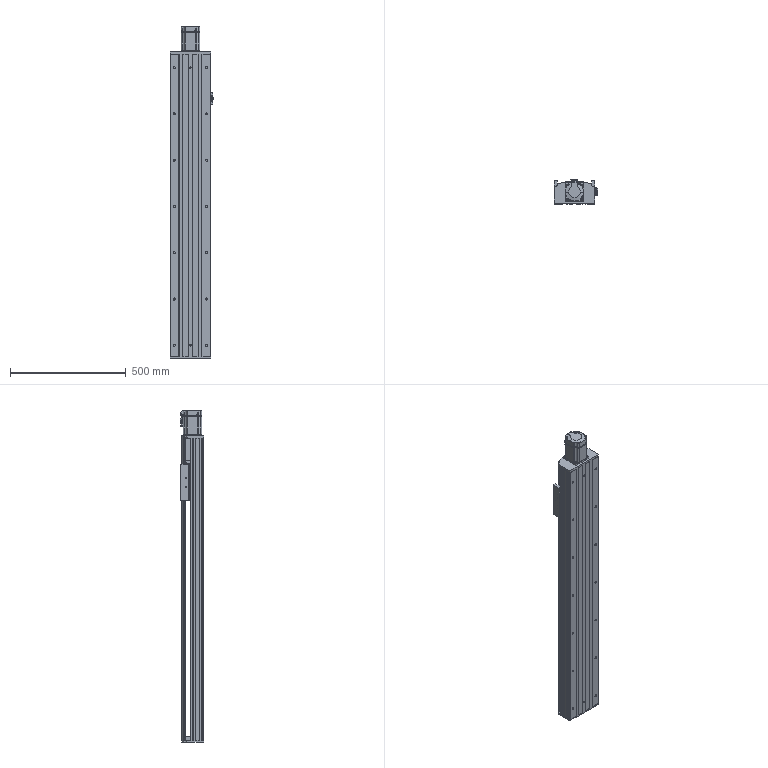Part | STEP file | TPA-HNR-175D-2510C-L1000-M-C-P75-N3 | 8 solids | 1594 faces | box 188.7 x 103 x 1435 mm | volume 7507272 mm3 | plane 788 | cylinder 613 | cone 175 | spline 18 | commonest cylinder face diameters 4.2 x88 10 x52 6 x47 8 x44 2.5 x36 5.5 x32